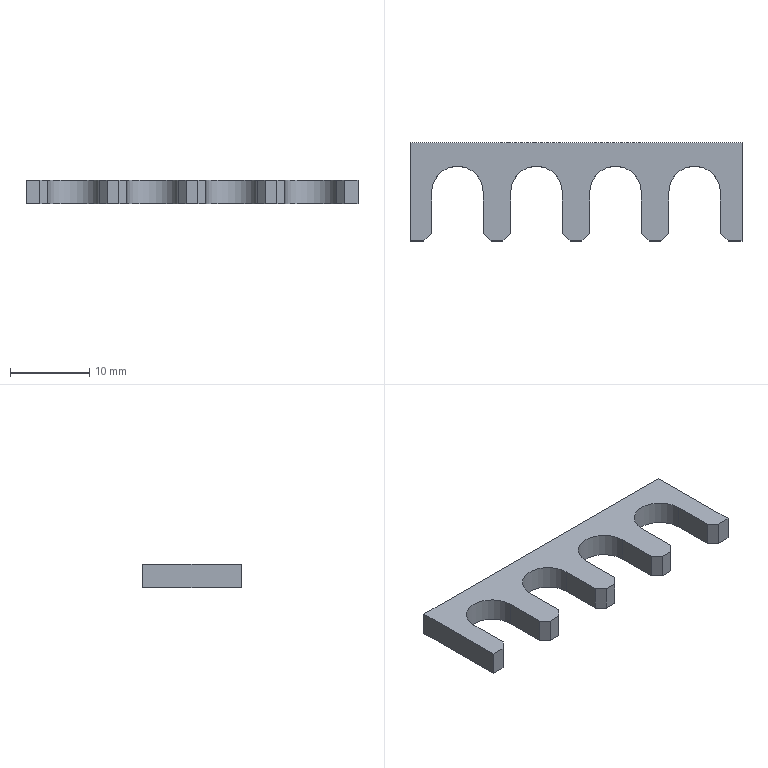Part | NX | features BREP 1 | 1 solid | 30 faces | box 42 x 12.4 x 3 mm | volume 867.702 mm3 | plane 26 | cylinder 4 | commonest cylinder face diameters 6.5 x4
STEP:
#1=CARTESIAN_POINT('',(-21.,0.,0.));
#2=VERTEX_POINT('',#1);
#3=CARTESIAN_POINT('',(-21.,-12.4,0.));
#4=VERTEX_POINT('',#3);
#5=CARTESIAN_POINT('',(-21.,-12.4,0.));
#6=DIRECTION('',(0.,-1.,0.));
#7=VECTOR('',#6,1000.);
#8=LINE('',#5,#7);
#9=EDGE_CURVE('',#2,#4,#8,.T.);
#10=ORIENTED_EDGE('',*,*,#9,.T.);
#11=CARTESIAN_POINT('',(-21.,-12.4,3.));
#12=VERTEX_POINT('',#11);
#13=CARTESIAN_POINT('',(-21.,-12.4,3.));
#14=DIRECTION('',(0.,0.,-1.));
#15=VECTOR('',#14,1000.);
#16=LINE('',#13,#15);
#17=EDGE_CURVE('',#12,#4,#16,.T.);
#18=ORIENTED_EDGE('',*,*,#17,.F.);
#19=CARTESIAN_POINT('',(-21.,0.,3.));
#20=VERTEX_POINT('',#19);
#21=CARTESIAN_POINT('',(-21.,-12.4,3.));
#22=DIRECTION('',(0.,-1.,0.));
#23=VECTOR('',#22,1000.);
#24=LINE('',#21,#23);
#25=EDGE_CURVE('',#20,#12,#24,.T.);
#26=ORIENTED_EDGE('',*,*,#25,.F.);
#27=CARTESIAN_POINT('',(-21.,0.,3.));
#28=DIRECTION('',(0.,0.,-1.));
#29=VECTOR('',#28,1000.);
#30=LINE('',#27,#29);
#31=EDGE_CURVE('',#20,#2,#30,.T.);
#32=ORIENTED_EDGE('',*,*,#31,.T.);
#33=EDGE_LOOP('',(#10,#18,#26,#32));
#34=FACE_BOUND('',#33,.T.);
#35=CARTESIAN_POINT('',(-21.,-12.4,3.));
#36=DIRECTION('',(1.,0.,0.));
#37=DIRECTION('',(0.,-1.,0.));
#38=AXIS2_PLACEMENT_3D('',#35,#36,#37);
#39=PLANE('',#38);
#40=ADVANCED_FACE('',(#34),#39,.F.);
#41=CARTESIAN_POINT('',(-19.25,-12.4,0.));
#42=VERTEX_POINT('',#41);
#43=CARTESIAN_POINT('',(-18.25,-12.4,0.));
#44=DIRECTION('',(1.,0.,0.));
#45=VECTOR('',#44,1000.);
#46=LINE('',#43,#45);
#47=EDGE_CURVE('',#4,#42,#46,.T.);
#48=ORIENTED_EDGE('',*,*,#47,.T.);
#49=CARTESIAN_POINT('',(-19.25,-12.4,3.));
#50=VERTEX_POINT('',#49);
#51=CARTESIAN_POINT('',(-19.25,-12.4,3.));
#52=DIRECTION('',(0.,0.,1.));
#53=VECTOR('',#52,1000.);
#54=LINE('',#51,#53);
#55=EDGE_CURVE('',#42,#50,#54,.T.);
#56=ORIENTED_EDGE('',*,*,#55,.T.);
#57=CARTESIAN_POINT('',(-18.25,-12.4,3.));
#58=DIRECTION('',(1.,0.,0.));
#59=VECTOR('',#58,1000.);
#60=LINE('',#57,#59);
#61=EDGE_CURVE('',#12,#50,#60,.T.);
#62=ORIENTED_EDGE('',*,*,#61,.F.);
#63=ORIENTED_EDGE('',*,*,#17,.T.);
#64=EDGE_LOOP('',(#48,#56,#62,#63));
#65=FACE_BOUND('',#64,.T.);
#66=CARTESIAN_POINT('',(-18.25,-12.4,3.));
#67=DIRECTION('',(0.,1.,0.));
#68=DIRECTION('',(0.,0.,-1.));
#69=AXIS2_PLACEMENT_3D('',#66,#67,#68);
#70=PLANE('',#69);
#71=ADVANCED_FACE('',(#65),#70,.F.);
#72=CARTESIAN_POINT('',(-18.25,-11.4,3.));
#73=VERTEX_POINT('',#72);
#74=CARTESIAN_POINT('',(-18.25,-6.2,3.));
#75=VERTEX_POINT('',#74);
#76=CARTESIAN_POINT('',(-18.25,-6.2,3.));
#77=DIRECTION('',(0.,1.,0.));
#78=VECTOR('',#77,1000.);
#79=LINE('',#76,#78);
#80=EDGE_CURVE('',#73,#75,#79,.T.);
#81=ORIENTED_EDGE('',*,*,#80,.F.);
#82=CARTESIAN_POINT('',(-18.25,-11.4,0.));
#83=VERTEX_POINT('',#82);
#84=CARTESIAN_POINT('',(-18.25,-11.4,3.));
#85=DIRECTION('',(0.,0.,-1.));
#86=VECTOR('',#85,1000.);
#87=LINE('',#84,#86);
#88=EDGE_CURVE('',#73,#83,#87,.T.);
#89=ORIENTED_EDGE('',*,*,#88,.T.);
#90=CARTESIAN_POINT('',(-18.25,-6.2,0.));
#91=VERTEX_POINT('',#90);
#92=CARTESIAN_POINT('',(-18.25,-6.2,0.));
#93=DIRECTION('',(0.,1.,0.));
#94=VECTOR('',#93,1000.);
#95=LINE('',#92,#94);
#96=EDGE_CURVE('',#83,#91,#95,.T.);
#97=ORIENTED_EDGE('',*,*,#96,.T.);
#98=CARTESIAN_POINT('',(-18.25,-6.2,3.));
#99=DIRECTION('',(0.,0.,-1.));
#100=VECTOR('',#99,1000.);
#101=LINE('',#98,#100);
#102=EDGE_CURVE('',#75,#91,#101,.T.);
#103=ORIENTED_EDGE('',*,*,#102,.F.);
#104=EDGE_LOOP('',(#81,#89,#97,#103));
#105=FACE_BOUND('',#104,.T.);
#106=CARTESIAN_POINT('',(-18.25,-6.2,3.));
#107=DIRECTION('',(-1.,0.,0.));
#108=DIRECTION('',(0.,1.,0.));
#109=AXIS2_PLACEMENT_3D('',#106,#107,#108);
#110=PLANE('',#109);
#111=ADVANCED_FACE('',(#105),#110,.F.);
#112=CARTESIAN_POINT('',(-11.75,-6.2,0.));
#113=VERTEX_POINT('',#112);
#114=CARTESIAN_POINT('',(-15.,-6.2,0.));
#115=DIRECTION('',(0.,0.,-1.));
#116=DIRECTION('',(1.,0.,0.));
#117=AXIS2_PLACEMENT_3D('',#114,#115,#116);
#118=CIRCLE('',#117,3.25);
#119=EDGE_CURVE('',#91,#113,#118,.T.);
#120=ORIENTED_EDGE('',*,*,#119,.T.);
#121=CARTESIAN_POINT('',(-11.75,-6.2,3.));
#122=VERTEX_POINT('',#121);
#123=CARTESIAN_POINT('',(-11.75,-6.2,3.));
#124=DIRECTION('',(0.,0.,-1.));
#125=VECTOR('',#124,1000.);
#126=LINE('',#123,#125);
#127=EDGE_CURVE('',#122,#113,#126,.T.);
#128=ORIENTED_EDGE('',*,*,#127,.F.);
#129=CARTESIAN_POINT('',(-15.,-6.2,3.));
#130=DIRECTION('',(0.,0.,-1.));
#131=DIRECTION('',(1.,0.,0.));
#132=AXIS2_PLACEMENT_3D('',#129,#130,#131);
#133=CIRCLE('',#132,3.25);
#134=EDGE_CURVE('',#75,#122,#133,.T.);
#135=ORIENTED_EDGE('',*,*,#134,.F.);
#136=ORIENTED_EDGE('',*,*,#102,.T.);
#137=EDGE_LOOP('',(#120,#128,#135,#136));
#138=FACE_BOUND('',#137,.T.);
#139=CARTESIAN_POINT('',(-15.,-6.2,3.));
#140=DIRECTION('',(0.,0.,-1.));
#141=DIRECTION('',(1.,0.,0.));
#142=AXIS2_PLACEMENT_3D('',#139,#140,#141);
#143=CYLINDRICAL_SURFACE('',#142,3.25);
#144=ADVANCED_FACE('',(#138),#143,.F.);
#145=CARTESIAN_POINT('',(-11.75,-11.4,0.));
#146=VERTEX_POINT('',#145);
#147=CARTESIAN_POINT('',(-11.75,-12.4,0.));
#148=DIRECTION('',(0.,-1.,0.));
#149=VECTOR('',#148,1000.);
#150=LINE('',#147,#149);
#151=EDGE_CURVE('',#113,#146,#150,.T.);
#152=ORIENTED_EDGE('',*,*,#151,.T.);
#153=CARTESIAN_POINT('',(-11.75,-11.4,3.));
#154=VERTEX_POINT('',#153);
#155=CARTESIAN_POINT('',(-11.75,-11.4,3.));
#156=DIRECTION('',(0.,0.,1.));
#157=VECTOR('',#156,1000.);
#158=LINE('',#155,#157);
#159=EDGE_CURVE('',#146,#154,#158,.T.);
#160=ORIENTED_EDGE('',*,*,#159,.T.);
#161=CARTESIAN_POINT('',(-11.75,-12.4,3.));
#162=DIRECTION('',(0.,-1.,0.));
#163=VECTOR('',#162,1000.);
#164=LINE('',#161,#163);
#165=EDGE_CURVE('',#122,#154,#164,.T.);
#166=ORIENTED_EDGE('',*,*,#165,.F.);
#167=ORIENTED_EDGE('',*,*,#127,.T.);
#168=EDGE_LOOP('',(#152,#160,#166,#167));
#169=FACE_BOUND('',#168,.T.);
#170=CARTESIAN_POINT('',(-11.75,-12.4,3.));
#171=DIRECTION('',(1.,0.,0.));
#172=DIRECTION('',(0.,0.,1.));
#173=AXIS2_PLACEMENT_3D('',#170,#171,#172);
#174=PLANE('',#173);
#175=ADVANCED_FACE('',(#169),#174,.F.);
#176=CARTESIAN_POINT('',(-10.75,-12.4,3.));
#177=VERTEX_POINT('',#176);
#178=CARTESIAN_POINT('',(-9.25,-12.4,3.));
#179=VERTEX_POINT('',#178);
#180=CARTESIAN_POINT('',(-8.25,-12.4,3.));
#181=DIRECTION('',(1.,0.,0.));
#182=VECTOR('',#181,1000.);
#183=LINE('',#180,#182);
#184=EDGE_CURVE('',#177,#179,#183,.T.);
#185=ORIENTED_EDGE('',*,*,#184,.F.);
#186=CARTESIAN_POINT('',(-10.75,-12.4,0.));
#187=VERTEX_POINT('',#186);
#188=CARTESIAN_POINT('',(-10.75,-12.4,3.));
#189=DIRECTION('',(0.,0.,-1.));
#190=VECTOR('',#189,1000.);
#191=LINE('',#188,#190);
#192=EDGE_CURVE('',#177,#187,#191,.T.);
#193=ORIENTED_EDGE('',*,*,#192,.T.);
#194=CARTESIAN_POINT('',(-9.25,-12.4,0.));
#195=VERTEX_POINT('',#194);
#196=CARTESIAN_POINT('',(-8.25,-12.4,0.));
#197=DIRECTION('',(1.,0.,0.));
#198=VECTOR('',#197,1000.);
#199=LINE('',#196,#198);
#200=EDGE_CURVE('',#187,#195,#199,.T.);
#201=ORIENTED_EDGE('',*,*,#200,.T.);
#202=CARTESIAN_POINT('',(-9.25,-12.4,3.));
#203=DIRECTION('',(0.,0.,1.));
#204=VECTOR('',#203,1000.);
#205=LINE('',#202,#204);
#206=EDGE_CURVE('',#195,#179,#205,.T.);
#207=ORIENTED_EDGE('',*,*,#206,.T.);
#208=EDGE_LOOP('',(#185,#193,#201,#207));
#209=FACE_BOUND('',#208,.T.);
#210=CARTESIAN_POINT('',(-8.25,-12.4,3.));
#211=DIRECTION('',(0.,1.,0.));
#212=DIRECTION('',(0.,0.,-1.));
#213=AXIS2_PLACEMENT_3D('',#210,#211,#212);
#214=PLANE('',#213);
#215=ADVANCED_FACE('',(#209),#214,.F.);
#216=CARTESIAN_POINT('',(-8.25,-11.4,3.));
#217=VERTEX_POINT('',#216);
#218=CARTESIAN_POINT('',(-8.25,-6.2,3.));
#219=VERTEX_POINT('',#218);
#220=CARTESIAN_POINT('',(-8.25,-6.2,3.));
#221=DIRECTION('',(0.,1.,0.));
#222=VECTOR('',#221,1000.);
#223=LINE('',#220,#222);
#224=EDGE_CURVE('',#217,#219,#223,.T.);
#225=ORIENTED_EDGE('',*,*,#224,.F.);
#226=CARTESIAN_POINT('',(-8.25,-11.4,0.));
#227=VERTEX_POINT('',#226);
#228=CARTESIAN_POINT('',(-8.25,-11.4,3.));
#229=DIRECTION('',(0.,0.,-1.));
#230=VECTOR('',#229,1000.);
#231=LINE('',#228,#230);
#232=EDGE_CURVE('',#217,#227,#231,.T.);
#233=ORIENTED_EDGE('',*,*,#232,.T.);
#234=CARTESIAN_POINT('',(-8.25,-6.2,0.));
#235=VERTEX_POINT('',#234);
#236=CARTESIAN_POINT('',(-8.25,-6.2,0.));
#237=DIRECTION('',(0.,1.,0.));
#238=VECTOR('',#237,1000.);
#239=LINE('',#236,#238);
#240=EDGE_CURVE('',#227,#235,#239,.T.);
#241=ORIENTED_EDGE('',*,*,#240,.T.);
#242=CARTESIAN_POINT('',(-8.25,-6.2,3.));
#243=DIRECTION('',(0.,0.,-1.));
#244=VECTOR('',#243,1000.);
#245=LINE('',#242,#244);
#246=EDGE_CURVE('',#219,#235,#245,.T.);
#247=ORIENTED_EDGE('',*,*,#246,.F.);
#248=EDGE_LOOP('',(#225,#233,#241,#247));
#249=FACE_BOUND('',#248,.T.);
#250=CARTESIAN_POINT('',(-8.25,-6.2,3.));
#251=DIRECTION('',(-1.,0.,0.));
#252=DIRECTION('',(0.,1.,0.));
#253=AXIS2_PLACEMENT_3D('',#250,#251,#252);
#254=PLANE('',#253);
#255=ADVANCED_FACE('',(#249),#254,.F.);
#256=CARTESIAN_POINT('',(-1.75,-6.2,0.));
#257=VERTEX_POINT('',#256);
#258=CARTESIAN_POINT('',(-5.,-6.2,0.));
#259=DIRECTION('',(0.,0.,-1.));
#260=DIRECTION('',(1.,0.,0.));
#261=AXIS2_PLACEMENT_3D('',#258,#259,#260);
#262=CIRCLE('',#261,3.25);
#263=EDGE_CURVE('',#235,#257,#262,.T.);
#264=ORIENTED_EDGE('',*,*,#263,.T.);
#265=CARTESIAN_POINT('',(-1.75,-6.2,3.));
#266=VERTEX_POINT('',#265);
#267=CARTESIAN_POINT('',(-1.75,-6.2,3.));
#268=DIRECTION('',(0.,0.,-1.));
#269=VECTOR('',#268,1000.);
#270=LINE('',#267,#269);
#271=EDGE_CURVE('',#266,#257,#270,.T.);
#272=ORIENTED_EDGE('',*,*,#271,.F.);
#273=CARTESIAN_POINT('',(-5.,-6.2,3.));
#274=DIRECTION('',(0.,0.,-1.));
#275=DIRECTION('',(1.,0.,0.));
#276=AXIS2_PLACEMENT_3D('',#273,#274,#275);
#277=CIRCLE('',#276,3.25);
#278=EDGE_CURVE('',#219,#266,#277,.T.);
#279=ORIENTED_EDGE('',*,*,#278,.F.);
#280=ORIENTED_EDGE('',*,*,#246,.T.);
#281=EDGE_LOOP('',(#264,#272,#279,#280));
#282=FACE_BOUND('',#281,.T.);
#283=CARTESIAN_POINT('',(-5.,-6.2,3.));
#284=DIRECTION('',(0.,0.,-1.));
#285=DIRECTION('',(1.,0.,0.));
#286=AXIS2_PLACEMENT_3D('',#283,#284,#285);
#287=CYLINDRICAL_SURFACE('',#286,3.25);
#288=ADVANCED_FACE('',(#282),#287,.F.);
#289=CARTESIAN_POINT('',(-1.75,-11.4,0.));
#290=VERTEX_POINT('',#289);
#291=CARTESIAN_POINT('',(-1.75,-12.4,0.));
#292=DIRECTION('',(0.,-1.,0.));
#293=VECTOR('',#292,1000.);
#294=LINE('',#291,#293);
#295=EDGE_CURVE('',#257,#290,#294,.T.);
#296=ORIENTED_EDGE('',*,*,#295,.T.);
#297=CARTESIAN_POINT('',(-1.75,-11.4,3.));
#298=VERTEX_POINT('',#297);
#299=CARTESIAN_POINT('',(-1.75,-11.4,3.));
#300=DIRECTION('',(0.,0.,1.));
#301=VECTOR('',#300,1000.);
#302=LINE('',#299,#301);
#303=EDGE_CURVE('',#290,#298,#302,.T.);
#304=ORIENTED_EDGE('',*,*,#303,.T.);
#305=CARTESIAN_POINT('',(-1.75,-12.4,3.));
#306=DIRECTION('',(0.,-1.,0.));
#307=VECTOR('',#306,1000.);
#308=LINE('',#305,#307);
#309=EDGE_CURVE('',#266,#298,#308,.T.);
#310=ORIENTED_EDGE('',*,*,#309,.F.);
#311=ORIENTED_EDGE('',*,*,#271,.T.);
#312=EDGE_LOOP('',(#296,#304,#310,#311));
#313=FACE_BOUND('',#312,.T.);
#314=CARTESIAN_POINT('',(-1.75,-12.4,3.));
#315=DIRECTION('',(1.,0.,0.));
#316=DIRECTION('',(0.,0.,1.));
#317=AXIS2_PLACEMENT_3D('',#314,#315,#316);
#318=PLANE('',#317);
#319=ADVANCED_FACE('',(#313),#318,.F.);
#320=CARTESIAN_POINT('',(-0.75,-12.4,3.));
#321=VERTEX_POINT('',#320);
#322=CARTESIAN_POINT('',(0.75,-12.4,3.));
#323=VERTEX_POINT('',#322);
#324=CARTESIAN_POINT('',(1.75,-12.4,3.));
#325=DIRECTION('',(1.,0.,0.));
#326=VECTOR('',#325,1000.);
#327=LINE('',#324,#326);
#328=EDGE_CURVE('',#321,#323,#327,.T.);
#329=ORIENTED_EDGE('',*,*,#328,.F.);
#330=CARTESIAN_POINT('',(-0.75,-12.4,0.));
#331=VERTEX_POINT('',#330);
#332=CARTESIAN_POINT('',(-0.75,-12.4,3.));
#333=DIRECTION('',(0.,0.,-1.));
#334=VECTOR('',#333,1000.);
#335=LINE('',#332,#334);
#336=EDGE_CURVE('',#321,#331,#335,.T.);
#337=ORIENTED_EDGE('',*,*,#336,.T.);
#338=CARTESIAN_POINT('',(0.75,-12.4,0.));
#339=VERTEX_POINT('',#338);
#340=CARTESIAN_POINT('',(1.75,-12.4,0.));
#341=DIRECTION('',(1.,0.,0.));
#342=VECTOR('',#341,1000.);
#343=LINE('',#340,#342);
#344=EDGE_CURVE('',#331,#339,#343,.T.);
#345=ORIENTED_EDGE('',*,*,#344,.T.);
#346=CARTESIAN_POINT('',(0.75,-12.4,3.));
#347=DIRECTION('',(0.,0.,1.));
#348=VECTOR('',#347,1000.);
#349=LINE('',#346,#348);
#350=EDGE_CURVE('',#339,#323,#349,.T.);
#351=ORIENTED_EDGE('',*,*,#350,.T.);
#352=EDGE_LOOP('',(#329,#337,#345,#351));
#353=FACE_BOUND('',#352,.T.);
#354=CARTESIAN_POINT('',(1.75,-12.4,3.));
#355=DIRECTION('',(0.,1.,0.));
#356=DIRECTION('',(0.,0.,-1.));
#357=AXIS2_PLACEMENT_3D('',#354,#355,#356);
#358=PLANE('',#357);
#359=ADVANCED_FACE('',(#353),#358,.F.);
#360=CARTESIAN_POINT('',(1.75,-11.4,3.));
#361=VERTEX_POINT('',#360);
#362=CARTESIAN_POINT('',(1.75,-6.2,3.));
#363=VERTEX_POINT('',#362);
#364=CARTESIAN_POINT('',(1.75,-6.2,3.));
#365=DIRECTION('',(0.,1.,0.));
#366=VECTOR('',#365,1000.);
#367=LINE('',#364,#366);
#368=EDGE_CURVE('',#361,#363,#367,.T.);
#369=ORIENTED_EDGE('',*,*,#368,.F.);
#370=CARTESIAN_POINT('',(1.75,-11.4,0.));
#371=VERTEX_POINT('',#370);
#372=CARTESIAN_POINT('',(1.75,-11.4,3.));
#373=DIRECTION('',(0.,0.,-1.));
#374=VECTOR('',#373,1000.);
#375=LINE('',#372,#374);
#376=EDGE_CURVE('',#361,#371,#375,.T.);
#377=ORIENTED_EDGE('',*,*,#376,.T.);
#378=CARTESIAN_POINT('',(1.75,-6.2,0.));
#379=VERTEX_POINT('',#378);
#380=CARTESIAN_POINT('',(1.75,-6.2,0.));
#381=DIRECTION('',(0.,1.,0.));
#382=VECTOR('',#381,1000.);
#383=LINE('',#380,#382);
#384=EDGE_CURVE('',#371,#379,#383,.T.);
#385=ORIENTED_EDGE('',*,*,#384,.T.);
#386=CARTESIAN_POINT('',(1.75,-6.2,3.));
#387=DIRECTION('',(0.,0.,-1.));
#388=VECTOR('',#387,1000.);
#389=LINE('',#386,#388);
#390=EDGE_CURVE('',#363,#379,#389,.T.);
#391=ORIENTED_EDGE('',*,*,#390,.F.);
#392=EDGE_LOOP('',(#369,#377,#385,#391));
#393=FACE_BOUND('',#392,.T.);
#394=CARTESIAN_POINT('',(1.75,-6.2,3.));
#395=DIRECTION('',(-1.,0.,0.));
#396=DIRECTION('',(0.,0.,-1.));
#397=AXIS2_PLACEMENT_3D('',#394,#395,#396);
#398=PLANE('',#397);
#399=ADVANCED_FACE('',(#393),#398,.F.);
#400=CARTESIAN_POINT('',(8.25,-6.2,0.));
#401=VERTEX_POINT('',#400);
#402=CARTESIAN_POINT('',(5.,-6.2,0.));
#403=DIRECTION('',(0.,0.,-1.));
#404=DIRECTION('',(1.,0.,0.));
#405=AXIS2_PLACEMENT_3D('',#402,#403,#404);
#406=CIRCLE('',#405,3.25);
#407=EDGE_CURVE('',#379,#401,#406,.T.);
#408=ORIENTED_EDGE('',*,*,#407,.T.);
#409=CARTESIAN_POINT('',(8.25,-6.2,3.));
#410=VERTEX_POINT('',#409);
#411=CARTESIAN_POINT('',(8.25,-6.2,3.));
#412=DIRECTION('',(0.,0.,-1.));
#413=VECTOR('',#412,1000.);
#414=LINE('',#411,#413);
#415=EDGE_CURVE('',#410,#401,#414,.T.);
#416=ORIENTED_EDGE('',*,*,#415,.F.);
#417=CARTESIAN_POINT('',(5.,-6.2,3.));
#418=DIRECTION('',(0.,0.,-1.));
#419=DIRECTION('',(1.,0.,0.));
#420=AXIS2_PLACEMENT_3D('',#417,#418,#419);
#421=CIRCLE('',#420,3.25);
#422=EDGE_CURVE('',#363,#410,#421,.T.);
#423=ORIENTED_EDGE('',*,*,#422,.F.);
#424=ORIENTED_EDGE('',*,*,#390,.T.);
#425=EDGE_LOOP('',(#408,#416,#423,#424));
#426=FACE_BOUND('',#425,.T.);
#427=CARTESIAN_POINT('',(5.,-6.2,3.));
#428=DIRECTION('',(0.,0.,-1.));
#429=DIRECTION('',(1.,0.,0.));
#430=AXIS2_PLACEMENT_3D('',#427,#428,#429);
#431=CYLINDRICAL_SURFACE('',#430,3.25);
#432=ADVANCED_FACE('',(#426),#431,.F.);
#433=CARTESIAN_POINT('',(8.25,-11.4,0.));
#434=VERTEX_POINT('',#433);
#435=CARTESIAN_POINT('',(8.25,-12.4,0.));
#436=DIRECTION('',(0.,-1.,0.));
#437=VECTOR('',#436,1000.);
#438=LINE('',#435,#437);
#439=EDGE_CURVE('',#401,#434,#438,.T.);
#440=ORIENTED_EDGE('',*,*,#439,.T.);
#441=CARTESIAN_POINT('',(8.25,-11.4,3.));
#442=VERTEX_POINT('',#441);
#443=CARTESIAN_POINT('',(8.25,-11.4,3.));
#444=DIRECTION('',(0.,0.,1.));
#445=VECTOR('',#444,1000.);
#446=LINE('',#443,#445);
#447=EDGE_CURVE('',#434,#442,#446,.T.);
#448=ORIENTED_EDGE('',*,*,#447,.T.);
#449=CARTESIAN_POINT('',(8.25,-12.4,3.));
#450=DIRECTION('',(0.,-1.,0.));
#451=VECTOR('',#450,1000.);
#452=LINE('',#449,#451);
#453=EDGE_CURVE('',#410,#442,#452,.T.);
#454=ORIENTED_EDGE('',*,*,#453,.F.);
#455=ORIENTED_EDGE('',*,*,#415,.T.);
#456=EDGE_LOOP('',(#440,#448,#454,#455));
#457=FACE_BOUND('',#456,.T.);
#458=CARTESIAN_POINT('',(8.25,-12.4,3.));
#459=DIRECTION('',(1.,0.,0.));
#460=DIRECTION('',(0.,-1.,0.));
#461=AXIS2_PLACEMENT_3D('',#458,#459,#460);
#462=PLANE('',#461);
#463=ADVANCED_FACE('',(#457),#462,.F.);
#464=CARTESIAN_POINT('',(9.25,-12.4,3.));
#465=VERTEX_POINT('',#464);
#466=CARTESIAN_POINT('',(10.75,-12.4,3.));
#467=VERTEX_POINT('',#466);
#468=CARTESIAN_POINT('',(11.75,-12.4,3.));
#469=DIRECTION('',(1.,0.,0.));
#470=VECTOR('',#469,1000.);
#471=LINE('',#468,#470);
#472=EDGE_CURVE('',#465,#467,#471,.T.);
#473=ORIENTED_EDGE('',*,*,#472,.F.);
#474=CARTESIAN_POINT('',(9.25,-12.4,0.));
#475=VERTEX_POINT('',#474);
#476=CARTESIAN_POINT('',(9.25,-12.4,3.));
#477=DIRECTION('',(0.,0.,-1.));
#478=VECTOR('',#477,1000.);
#479=LINE('',#476,#478);
#480=EDGE_CURVE('',#465,#475,#479,.T.);
#481=ORIENTED_EDGE('',*,*,#480,.T.);
#482=CARTESIAN_POINT('',(10.75,-12.4,0.));
#483=VERTEX_POINT('',#482);
#484=CARTESIAN_POINT('',(11.75,-12.4,0.));
#485=DIRECTION('',(1.,0.,0.));
#486=VECTOR('',#485,1000.);
#487=LINE('',#484,#486);
#488=EDGE_CURVE('',#475,#483,#487,.T.);
#489=ORIENTED_EDGE('',*,*,#488,.T.);
#490=CARTESIAN_POINT('',(10.75,-12.4,3.));
#491=DIRECTION('',(0.,0.,1.));
#492=VECTOR('',#491,1000.);
#493=LINE('',#490,#492);
#494=EDGE_CURVE('',#483,#467,#493,.T.);
#495=ORIENTED_EDGE('',*,*,#494,.T.);
#496=EDGE_LOOP('',(#473,#481,#489,#495));
#497=FACE_BOUND('',#496,.T.);
#498=CARTESIAN_POINT('',(11.75,-12.4,3.));
#499=DIRECTION('',(0.,1.,0.));
#500=DIRECTION('',(0.,0.,-1.));
#501=AXIS2_PLACEMENT_3D('',#498,#499,#500);
#502=PLANE('',#501);
#503=ADVANCED_FACE('',(#497),#502,.F.);
#504=CARTESIAN_POINT('',(11.75,-11.4,3.));
#505=VERTEX_POINT('',#504);
#506=CARTESIAN_POINT('',(11.75,-6.2,3.));
#507=VERTEX_POINT('',#506);
#508=CARTESIAN_POINT('',(11.75,-6.2,3.));
#509=DIRECTION('',(0.,1.,0.));
#510=VECTOR('',#509,1000.);
#511=LINE('',#508,#510);
#512=EDGE_CURVE('',#505,#507,#511,.T.);
#513=ORIENTED_EDGE('',*,*,#512,.F.);
#514=CARTESIAN_POINT('',(11.75,-11.4,0.));
#515=VERTEX_POINT('',#514);
#516=CARTESIAN_POINT('',(11.75,-11.4,3.));
#517=DIRECTION('',(0.,0.,-1.));
#518=VECTOR('',#517,1000.);
#519=LINE('',#516,#518);
#520=EDGE_CURVE('',#505,#515,#519,.T.);
#521=ORIENTED_EDGE('',*,*,#520,.T.);
#522=CARTESIAN_POINT('',(11.75,-6.2,0.));
#523=VERTEX_POINT('',#522);
#524=CARTESIAN_POINT('',(11.75,-6.2,0.));
#525=DIRECTION('',(0.,1.,0.));
#526=VECTOR('',#525,1000.);
#527=LINE('',#524,#526);
#528=EDGE_CURVE('',#515,#523,#527,.T.);
#529=ORIENTED_EDGE('',*,*,#528,.T.);
#530=CARTESIAN_POINT('',(11.75,-6.2,3.));
#531=DIRECTION('',(0.,0.,-1.));
#532=VECTOR('',#531,1000.);
#533=LINE('',#530,#532);
#534=EDGE_CURVE('',#507,#523,#533,.T.);
#535=ORIENTED_EDGE('',*,*,#534,.F.);
#536=EDGE_LOOP('',(#513,#521,#529,#535));
#537=FACE_BOUND('',#536,.T.);
#538=CARTESIAN_POINT('',(11.75,-6.2,3.));
#539=DIRECTION('',(-1.,0.,0.));
#540=DIRECTION('',(0.,0.,-1.));
#541=AXIS2_PLACEMENT_3D('',#538,#539,#540);
#542=PLANE('',#541);
#543=ADVANCED_FACE('',(#537),#542,.F.);
#544=CARTESIAN_POINT('',(18.25,-6.2,0.));
#545=VERTEX_POINT('',#544);
#546=CARTESIAN_POINT('',(15.,-6.2,0.));
#547=DIRECTION('',(0.,0.,-1.));
#548=DIRECTION('',(1.,0.,0.));
#549=AXIS2_PLACEMENT_3D('',#546,#547,#548);
#550=CIRCLE('',#549,3.25);
#551=EDGE_CURVE('',#523,#545,#550,.T.);
#552=ORIENTED_EDGE('',*,*,#551,.T.);
#553=CARTESIAN_POINT('',(18.25,-6.2,3.));
#554=VERTEX_POINT('',#553);
#555=CARTESIAN_POINT('',(18.25,-6.2,3.));
#556=DIRECTION('',(0.,0.,-1.));
#557=VECTOR('',#556,1000.);
#558=LINE('',#555,#557);
#559=EDGE_CURVE('',#554,#545,#558,.T.);
#560=ORIENTED_EDGE('',*,*,#559,.F.);
#561=CARTESIAN_POINT('',(15.,-6.2,3.));
#562=DIRECTION('',(0.,0.,-1.));
#563=DIRECTION('',(1.,0.,0.));
#564=AXIS2_PLACEMENT_3D('',#561,#562,#563);
#565=CIRCLE('',#564,3.25);
#566=EDGE_CURVE('',#507,#554,#565,.T.);
#567=ORIENTED_EDGE('',*,*,#566,.F.);
#568=ORIENTED_EDGE('',*,*,#534,.T.);
#569=EDGE_LOOP('',(#552,#560,#567,#568));
#570=FACE_BOUND('',#569,.T.);
#571=CARTESIAN_POINT('',(15.,-6.2,3.));
#572=DIRECTION('',(0.,0.,-1.));
#573=DIRECTION('',(1.,0.,0.));
#574=AXIS2_PLACEMENT_3D('',#571,#572,#573);
#575=CYLINDRICAL_SURFACE('',#574,3.25);
#576=ADVANCED_FACE('',(#570),#575,.F.);
#577=CARTESIAN_POINT('',(18.25,-11.4,0.));
#578=VERTEX_POINT('',#577);
#579=CARTESIAN_POINT('',(18.25,-12.4,0.));
#580=DIRECTION('',(0.,-1.,0.));
#581=VECTOR('',#580,1000.);
#582=LINE('',#579,#581);
#583=EDGE_CURVE('',#545,#578,#582,.T.);
#584=ORIENTED_EDGE('',*,*,#583,.T.);
#585=CARTESIAN_POINT('',(18.25,-11.4,3.));
#586=VERTEX_POINT('',#585);
#587=CARTESIAN_POINT('',(18.25,-11.4,3.));
#588=DIRECTION('',(0.,0.,1.));
#589=VECTOR('',#588,1000.);
#590=LINE('',#587,#589);
#591=EDGE_CURVE('',#578,#586,#590,.T.);
#592=ORIENTED_EDGE('',*,*,#591,.T.);
#593=CARTESIAN_POINT('',(18.25,-12.4,3.));
#594=DIRECTION('',(0.,-1.,0.));
#595=VECTOR('',#594,1000.);
#596=LINE('',#593,#595);
#597=EDGE_CURVE('',#554,#586,#596,.T.);
#598=ORIENTED_EDGE('',*,*,#597,.F.);
#599=ORIENTED_EDGE('',*,*,#559,.T.);
#600=EDGE_LOOP('',(#584,#592,#598,#599));
#601=FACE_BOUND('',#600,.T.);
#602=CARTESIAN_POINT('',(18.25,-12.4,3.));
#603=DIRECTION('',(1.,0.,0.));
#604=DIRECTION('',(0.,-1.,0.));
#605=AXIS2_PLACEMENT_3D('',#602,#603,#604);
#606=PLANE('',#605);
#607=ADVANCED_FACE('',(#601),#606,.F.);
#608=CARTESIAN_POINT('',(19.25,-12.4,3.));
#609=VERTEX_POINT('',#608);
#610=CARTESIAN_POINT('',(21.,-12.4,3.));
#611=VERTEX_POINT('',#610);
#612=CARTESIAN_POINT('',(21.,-12.4,3.));
#613=DIRECTION('',(1.,0.,0.));
#614=VECTOR('',#613,1000.);
#615=LINE('',#612,#614);
#616=EDGE_CURVE('',#609,#611,#615,.T.);
#617=ORIENTED_EDGE('',*,*,#616,.F.);
#618=CARTESIAN_POINT('',(19.25,-12.4,0.));
#619=VERTEX_POINT('',#618);
#620=CARTESIAN_POINT('',(19.25,-12.4,3.));
#621=DIRECTION('',(0.,0.,-1.));
#622=VECTOR('',#621,1000.);
#623=LINE('',#620,#622);
#624=EDGE_CURVE('',#609,#619,#623,.T.);
#625=ORIENTED_EDGE('',*,*,#624,.T.);
#626=CARTESIAN_POINT('',(21.,-12.4,0.));
#627=VERTEX_POINT('',#626);
#628=CARTESIAN_POINT('',(21.,-12.4,0.));
#629=DIRECTION('',(1.,0.,0.));
#630=VECTOR('',#629,1000.);
#631=LINE('',#628,#630);
#632=EDGE_CURVE('',#619,#627,#631,.T.);
#633=ORIENTED_EDGE('',*,*,#632,.T.);
#634=CARTESIAN_POINT('',(21.,-12.4,3.));
#635=DIRECTION('',(0.,0.,-1.));
#636=VECTOR('',#635,1000.);
#637=LINE('',#634,#636);
#638=EDGE_CURVE('',#611,#627,#637,.T.);
#639=ORIENTED_EDGE('',*,*,#638,.F.);
#640=EDGE_LOOP('',(#617,#625,#633,#639));
#641=FACE_BOUND('',#640,.T.);
#642=CARTESIAN_POINT('',(21.,-12.4,3.));
#643=DIRECTION('',(0.,1.,0.));
#644=DIRECTION('',(1.,0.,0.));
#645=AXIS2_PLACEMENT_3D('',#642,#643,#644);
#646=PLANE('',#645);
#647=ADVANCED_FACE('',(#641),#646,.F.);
#648=CARTESIAN_POINT('',(21.,0.,0.));
#649=VERTEX_POINT('',#648);
#650=CARTESIAN_POINT('',(21.,0.,0.));
#651=DIRECTION('',(0.,1.,0.));
#652=VECTOR('',#651,1000.);
#653=LINE('',#650,#652);
#654=EDGE_CURVE('',#627,#649,#653,.T.);
#655=ORIENTED_EDGE('',*,*,#654,.T.);
#656=CARTESIAN_POINT('',(21.,0.,3.));
#657=VERTEX_POINT('',#656);
#658=CARTESIAN_POINT('',(21.,0.,3.));
#659=DIRECTION('',(0.,0.,-1.));
#660=VECTOR('',#659,1000.);
#661=LINE('',#658,#660);
#662=EDGE_CURVE('',#657,#649,#661,.T.);
#663=ORIENTED_EDGE('',*,*,#662,.F.);
#664=CARTESIAN_POINT('',(21.,0.,3.));
#665=DIRECTION('',(0.,1.,0.));
#666=VECTOR('',#665,1000.);
#667=LINE('',#664,#666);
#668=EDGE_CURVE('',#611,#657,#667,.T.);
#669=ORIENTED_EDGE('',*,*,#668,.F.);
#670=ORIENTED_EDGE('',*,*,#638,.T.);
#671=EDGE_LOOP('',(#655,#663,#669,#670));
#672=FACE_BOUND('',#671,.T.);
#673=CARTESIAN_POINT('',(21.,0.,3.));
#674=DIRECTION('',(-1.,0.,0.));
#675=DIRECTION('',(0.,1.,0.));
#676=AXIS2_PLACEMENT_3D('',#673,#674,#675);
#677=PLANE('',#676);
#678=ADVANCED_FACE('',(#672),#677,.F.);
#679=CARTESIAN_POINT('',(-21.,0.,0.));
#680=DIRECTION('',(-1.,0.,0.));
#681=VECTOR('',#680,1000.);
#682=LINE('',#679,#681);
#683=EDGE_CURVE('',#649,#2,#682,.T.);
#684=ORIENTED_EDGE('',*,*,#683,.T.);
#685=ORIENTED_EDGE('',*,*,#31,.F.);
#686=CARTESIAN_POINT('',(-21.,0.,3.));
#687=DIRECTION('',(-1.,0.,0.));
#688=VECTOR('',#687,1000.);
#689=LINE('',#686,#688);
#690=EDGE_CURVE('',#657,#20,#689,.T.);
#691=ORIENTED_EDGE('',*,*,#690,.F.);
#692=ORIENTED_EDGE('',*,*,#662,.T.);
#693=EDGE_LOOP('',(#684,#685,#691,#692));
#694=FACE_BOUND('',#693,.T.);
#695=CARTESIAN_POINT('',(-21.,0.,3.));
#696=DIRECTION('',(0.,-1.,0.));
#697=DIRECTION('',(-1.,0.,0.));
#698=AXIS2_PLACEMENT_3D('',#695,#696,#697);
#699=PLANE('',#698);
#700=ADVANCED_FACE('',(#694),#699,.F.);
#701=ORIENTED_EDGE('',*,*,#597,.T.);
#702=CARTESIAN_POINT('',(14.025,-7.175,3.));
#703=DIRECTION('',(0.7071,-0.7071,0.));
#704=VECTOR('',#703,1000.);
#705=LINE('',#702,#704);
#706=EDGE_CURVE('',#586,#609,#705,.T.);
#707=ORIENTED_EDGE('',*,*,#706,.T.);
#708=ORIENTED_EDGE('',*,*,#616,.T.);
#709=ORIENTED_EDGE('',*,*,#668,.T.);
#710=ORIENTED_EDGE('',*,*,#690,.T.);
#711=ORIENTED_EDGE('',*,*,#25,.T.);
#712=ORIENTED_EDGE('',*,*,#61,.T.);
#713=CARTESIAN_POINT('',(0.975,7.825,3.));
#714=DIRECTION('',(0.7071,0.7071,0.));
#715=VECTOR('',#714,1000.);
#716=LINE('',#713,#715);
#717=EDGE_CURVE('',#50,#73,#716,.T.);
#718=ORIENTED_EDGE('',*,*,#717,.T.);
#719=ORIENTED_EDGE('',*,*,#80,.T.);
#720=ORIENTED_EDGE('',*,*,#134,.T.);
#721=ORIENTED_EDGE('',*,*,#165,.T.);
#722=CARTESIAN_POINT('',(-0.975,-22.175,3.));
#723=DIRECTION('',(0.7071,-0.7071,0.));
#724=VECTOR('',#723,1000.);
#725=LINE('',#722,#724);
#726=EDGE_CURVE('',#154,#177,#725,.T.);
#727=ORIENTED_EDGE('',*,*,#726,.T.);
#728=ORIENTED_EDGE('',*,*,#184,.T.);
#729=CARTESIAN_POINT('',(5.975,2.825,3.));
#730=DIRECTION('',(0.7071,0.7071,0.));
#731=VECTOR('',#730,1000.);
#732=LINE('',#729,#731);
#733=EDGE_CURVE('',#179,#217,#732,.T.);
#734=ORIENTED_EDGE('',*,*,#733,.T.);
#735=ORIENTED_EDGE('',*,*,#224,.T.);
#736=ORIENTED_EDGE('',*,*,#278,.T.);
#737=ORIENTED_EDGE('',*,*,#309,.T.);
#738=CARTESIAN_POINT('',(4.025,-17.175,3.));
#739=DIRECTION('',(0.7071,-0.7071,0.));
#740=VECTOR('',#739,1000.);
#741=LINE('',#738,#740);
#742=EDGE_CURVE('',#298,#321,#741,.T.);
#743=ORIENTED_EDGE('',*,*,#742,.T.);
#744=ORIENTED_EDGE('',*,*,#328,.T.);
#745=CARTESIAN_POINT('',(10.975,-2.175,3.));
#746=DIRECTION('',(0.7071,0.7071,0.));
#747=VECTOR('',#746,1000.);
#748=LINE('',#745,#747);
#749=EDGE_CURVE('',#323,#361,#748,.T.);
#750=ORIENTED_EDGE('',*,*,#749,.T.);
#751=ORIENTED_EDGE('',*,*,#368,.T.);
#752=ORIENTED_EDGE('',*,*,#422,.T.);
#753=ORIENTED_EDGE('',*,*,#453,.T.);
#754=CARTESIAN_POINT('',(9.025,-12.175,3.));
#755=DIRECTION('',(0.7071,-0.7071,0.));
#756=VECTOR('',#755,1000.);
#757=LINE('',#754,#756);
#758=EDGE_CURVE('',#442,#465,#757,.T.);
#759=ORIENTED_EDGE('',*,*,#758,.T.);
#760=ORIENTED_EDGE('',*,*,#472,.T.);
#761=CARTESIAN_POINT('',(15.975,-7.175,3.));
#762=DIRECTION('',(0.7071,0.7071,0.));
#763=VECTOR('',#762,1000.);
#764=LINE('',#761,#763);
#765=EDGE_CURVE('',#467,#505,#764,.T.);
#766=ORIENTED_EDGE('',*,*,#765,.T.);
#767=ORIENTED_EDGE('',*,*,#512,.T.);
#768=ORIENTED_EDGE('',*,*,#566,.T.);
#769=EDGE_LOOP('',(#701,#707,#708,#709,#710,#711,#712,#718,#719,#720,#721,#727,#728,#734,#735,#736,#737,#743,#744,#750,#751,#752,#753,#759,#760,#766,#767,#768));
#770=FACE_BOUND('',#769,.T.);
#771=CARTESIAN_POINT('',(15.,-6.2,3.));
#772=DIRECTION('',(0.,0.,1.));
#773=DIRECTION('',(-1.,0.,0.));
#774=AXIS2_PLACEMENT_3D('',#771,#772,#773);
#775=PLANE('',#774);
#776=ADVANCED_FACE('',(#770),#775,.T.);
#777=ORIENTED_EDGE('',*,*,#632,.F.);
#778=CARTESIAN_POINT('',(19.25,-12.4,0.));
#779=DIRECTION('',(-0.7071,0.7071,0.));
#780=VECTOR('',#779,1000.);
#781=LINE('',#778,#780);
#782=EDGE_CURVE('',#619,#578,#781,.T.);
#783=ORIENTED_EDGE('',*,*,#782,.T.);
#784=ORIENTED_EDGE('',*,*,#583,.F.);
#785=ORIENTED_EDGE('',*,*,#551,.F.);
#786=ORIENTED_EDGE('',*,*,#528,.F.);
#787=CARTESIAN_POINT('',(11.75,-11.4,0.));
#788=DIRECTION('',(-0.7071,-0.7071,0.));
#789=VECTOR('',#788,1000.);
#790=LINE('',#787,#789);
#791=EDGE_CURVE('',#515,#483,#790,.T.);
#792=ORIENTED_EDGE('',*,*,#791,.T.);
#793=ORIENTED_EDGE('',*,*,#488,.F.);
#794=CARTESIAN_POINT('',(9.25,-12.4,0.));
#795=DIRECTION('',(-0.7071,0.7071,0.));
#796=VECTOR('',#795,1000.);
#797=LINE('',#794,#796);
#798=EDGE_CURVE('',#475,#434,#797,.T.);
#799=ORIENTED_EDGE('',*,*,#798,.T.);
#800=ORIENTED_EDGE('',*,*,#439,.F.);
#801=ORIENTED_EDGE('',*,*,#407,.F.);
#802=ORIENTED_EDGE('',*,*,#384,.F.);
#803=CARTESIAN_POINT('',(1.75,-11.4,0.));
#804=DIRECTION('',(-0.7071,-0.7071,0.));
#805=VECTOR('',#804,1000.);
#806=LINE('',#803,#805);
#807=EDGE_CURVE('',#371,#339,#806,.T.);
#808=ORIENTED_EDGE('',*,*,#807,.T.);
#809=ORIENTED_EDGE('',*,*,#344,.F.);
#810=CARTESIAN_POINT('',(-0.75,-12.4,0.));
#811=DIRECTION('',(-0.7071,0.7071,0.));
#812=VECTOR('',#811,1000.);
#813=LINE('',#810,#812);
#814=EDGE_CURVE('',#331,#290,#813,.T.);
#815=ORIENTED_EDGE('',*,*,#814,.T.);
#816=ORIENTED_EDGE('',*,*,#295,.F.);
#817=ORIENTED_EDGE('',*,*,#263,.F.);
#818=ORIENTED_EDGE('',*,*,#240,.F.);
#819=CARTESIAN_POINT('',(-8.25,-11.4,0.));
#820=DIRECTION('',(-0.7071,-0.7071,0.));
#821=VECTOR('',#820,1000.);
#822=LINE('',#819,#821);
#823=EDGE_CURVE('',#227,#195,#822,.T.);
#824=ORIENTED_EDGE('',*,*,#823,.T.);
#825=ORIENTED_EDGE('',*,*,#200,.F.);
#826=CARTESIAN_POINT('',(-10.75,-12.4,0.));
#827=DIRECTION('',(-0.7071,0.7071,0.));
#828=VECTOR('',#827,1000.);
#829=LINE('',#826,#828);
#830=EDGE_CURVE('',#187,#146,#829,.T.);
#831=ORIENTED_EDGE('',*,*,#830,.T.);
#832=ORIENTED_EDGE('',*,*,#151,.F.);
#833=ORIENTED_EDGE('',*,*,#119,.F.);
#834=ORIENTED_EDGE('',*,*,#96,.F.);
#835=CARTESIAN_POINT('',(-18.25,-11.4,0.));
#836=DIRECTION('',(-0.7071,-0.7071,0.));
#837=VECTOR('',#836,1000.);
#838=LINE('',#835,#837);
#839=EDGE_CURVE('',#83,#42,#838,.T.);
#840=ORIENTED_EDGE('',*,*,#839,.T.);
#841=ORIENTED_EDGE('',*,*,#47,.F.);
#842=ORIENTED_EDGE('',*,*,#9,.F.);
#843=ORIENTED_EDGE('',*,*,#683,.F.);
#844=ORIENTED_EDGE('',*,*,#654,.F.);
#845=EDGE_LOOP('',(#777,#783,#784,#785,#786,#792,#793,#799,#800,#801,#802,#808,#809,#815,#816,#817,#818,#824,#825,#831,#832,#833,#834,#840,#841,#842,#843,#844));
#846=FACE_BOUND('',#845,.T.);
#847=CARTESIAN_POINT('',(15.,-6.2,0.));
#848=DIRECTION('',(0.,0.,1.));
#849=DIRECTION('',(-1.,0.,0.));
#850=AXIS2_PLACEMENT_3D('',#847,#848,#849);
#851=PLANE('',#850);
#852=ADVANCED_FACE('',(#846),#851,.F.);
#853=ORIENTED_EDGE('',*,*,#706,.F.);
#854=ORIENTED_EDGE('',*,*,#591,.F.);
#855=ORIENTED_EDGE('',*,*,#782,.F.);
#856=ORIENTED_EDGE('',*,*,#624,.F.);
#857=EDGE_LOOP('',(#853,#854,#855,#856));
#858=FACE_BOUND('',#857,.T.);
#859=CARTESIAN_POINT('',(19.25,-12.4,3.));
#860=DIRECTION('',(0.7071,0.7071,0.));
#861=DIRECTION('',(0.,0.,1.));
#862=AXIS2_PLACEMENT_3D('',#859,#860,#861);
#863=PLANE('',#862);
#864=ADVANCED_FACE('',(#858),#863,.F.);
#865=ORIENTED_EDGE('',*,*,#758,.F.);
#866=ORIENTED_EDGE('',*,*,#447,.F.);
#867=ORIENTED_EDGE('',*,*,#798,.F.);
#868=ORIENTED_EDGE('',*,*,#480,.F.);
#869=EDGE_LOOP('',(#865,#866,#867,#868));
#870=FACE_BOUND('',#869,.T.);
#871=CARTESIAN_POINT('',(9.25,-12.4,3.));
#872=DIRECTION('',(0.7071,0.7071,0.));
#873=DIRECTION('',(0.,0.,1.));
#874=AXIS2_PLACEMENT_3D('',#871,#872,#873);
#875=PLANE('',#874);
#876=ADVANCED_FACE('',(#870),#875,.F.);
#877=ORIENTED_EDGE('',*,*,#742,.F.);
#878=ORIENTED_EDGE('',*,*,#303,.F.);
#879=ORIENTED_EDGE('',*,*,#814,.F.);
#880=ORIENTED_EDGE('',*,*,#336,.F.);
#881=EDGE_LOOP('',(#877,#878,#879,#880));
#882=FACE_BOUND('',#881,.T.);
#883=CARTESIAN_POINT('',(-0.75,-12.4,3.));
#884=DIRECTION('',(0.7071,0.7071,0.));
#885=DIRECTION('',(0.,0.,1.));
#886=AXIS2_PLACEMENT_3D('',#883,#884,#885);
#887=PLANE('',#886);
#888=ADVANCED_FACE('',(#882),#887,.F.);
#889=ORIENTED_EDGE('',*,*,#726,.F.);
#890=ORIENTED_EDGE('',*,*,#159,.F.);
#891=ORIENTED_EDGE('',*,*,#830,.F.);
#892=ORIENTED_EDGE('',*,*,#192,.F.);
#893=EDGE_LOOP('',(#889,#890,#891,#892));
#894=FACE_BOUND('',#893,.T.);
#895=CARTESIAN_POINT('',(-10.75,-12.4,3.));
#896=DIRECTION('',(0.7071,0.7071,0.));
#897=DIRECTION('',(0.,0.,1.));
#898=AXIS2_PLACEMENT_3D('',#895,#896,#897);
#899=PLANE('',#898);
#900=ADVANCED_FACE('',(#894),#899,.F.);
#901=ORIENTED_EDGE('',*,*,#765,.F.);
#902=ORIENTED_EDGE('',*,*,#494,.F.);
#903=ORIENTED_EDGE('',*,*,#791,.F.);
#904=ORIENTED_EDGE('',*,*,#520,.F.);
#905=EDGE_LOOP('',(#901,#902,#903,#904));
#906=FACE_BOUND('',#905,.T.);
#907=CARTESIAN_POINT('',(11.75,-11.4,3.));
#908=DIRECTION('',(-0.7071,0.7071,0.));
#909=DIRECTION('',(0.,0.,1.));
#910=AXIS2_PLACEMENT_3D('',#907,#908,#909);
#911=PLANE('',#910);
#912=ADVANCED_FACE('',(#906),#911,.F.);
#913=ORIENTED_EDGE('',*,*,#749,.F.);
#914=ORIENTED_EDGE('',*,*,#350,.F.);
#915=ORIENTED_EDGE('',*,*,#807,.F.);
#916=ORIENTED_EDGE('',*,*,#376,.F.);
#917=EDGE_LOOP('',(#913,#914,#915,#916));
#918=FACE_BOUND('',#917,.T.);
#919=CARTESIAN_POINT('',(1.75,-11.4,3.));
#920=DIRECTION('',(-0.7071,0.7071,0.));
#921=DIRECTION('',(0.,0.,1.));
#922=AXIS2_PLACEMENT_3D('',#919,#920,#921);
#923=PLANE('',#922);
#924=ADVANCED_FACE('',(#918),#923,.F.);
#925=ORIENTED_EDGE('',*,*,#717,.F.);
#926=ORIENTED_EDGE('',*,*,#55,.F.);
#927=ORIENTED_EDGE('',*,*,#839,.F.);
#928=ORIENTED_EDGE('',*,*,#88,.F.);
#929=EDGE_LOOP('',(#925,#926,#927,#928));
#930=FACE_BOUND('',#929,.T.);
#931=CARTESIAN_POINT('',(-18.25,-11.4,3.));
#932=DIRECTION('',(-0.7071,0.7071,0.));
#933=DIRECTION('',(0.,0.,1.));
#934=AXIS2_PLACEMENT_3D('',#931,#932,#933);
#935=PLANE('',#934);
#936=ADVANCED_FACE('',(#930),#935,.F.);
#937=ORIENTED_EDGE('',*,*,#733,.F.);
#938=ORIENTED_EDGE('',*,*,#206,.F.);
#939=ORIENTED_EDGE('',*,*,#823,.F.);
#940=ORIENTED_EDGE('',*,*,#232,.F.);
#941=EDGE_LOOP('',(#937,#938,#939,#940));
#942=FACE_BOUND('',#941,.T.);
#943=CARTESIAN_POINT('',(-8.25,-11.4,3.));
#944=DIRECTION('',(-0.7071,0.7071,0.));
#945=DIRECTION('',(0.,0.,1.));
#946=AXIS2_PLACEMENT_3D('',#943,#944,#945);
#947=PLANE('',#946);
#948=ADVANCED_FACE('',(#942),#947,.F.);
#949=CLOSED_SHELL('',(#40,#71,#111,#144,#175,#215,#255,#288,#319,#359,#399,#432,#463,#503,#543,#576,#607,#647,#678,#700,#776,#852,#864,#876,#888,#900,#912,#924,#936,#948));
#950=MANIFOLD_SOLID_BREP('',#949);
#951=(LENGTH_UNIT()NAMED_UNIT(*)SI_UNIT(.MILLI.,.METRE.));
#952=UNCERTAINTY_MEASURE_WITH_UNIT(LENGTH_MEASURE(0.00001),#951,'','');
#953=(NAMED_UNIT(*)PLANE_ANGLE_UNIT()SI_UNIT($,.RADIAN.));
#954=(NAMED_UNIT(*)SI_UNIT($,.STERADIAN.)SOLID_ANGLE_UNIT());
#955=(GEOMETRIC_REPRESENTATION_CONTEXT(3)GLOBAL_UNCERTAINTY_ASSIGNED_CONTEXT((#952))GLOBAL_UNIT_ASSIGNED_CONTEXT((#951,#953,#954))REPRESENTATION_CONTEXT('',''));
#956=ADVANCED_BREP_SHAPE_REPRESENTATION('',(#950),#955);